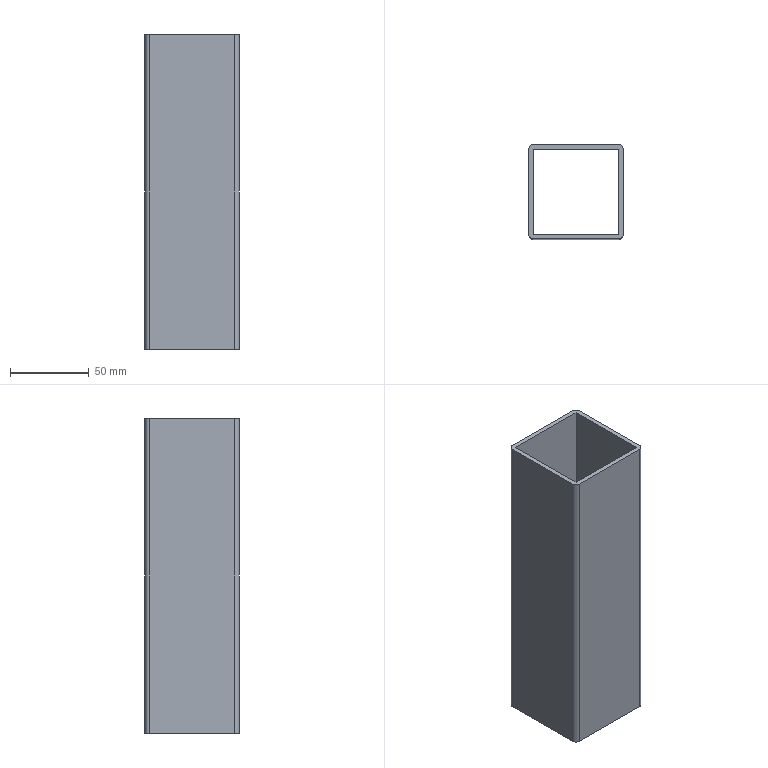Part | STEP file | X77-03109 | 1 solid | 14 faces | box 60 x 60 x 200 mm | volume 135255 mm3 | plane 10 | cylinder 4 | commonest cylinder face diameters 6 x4
STEP:
#1=CARTESIAN_POINT('',(0.,3.,200.));
#2=VERTEX_POINT('',#1);
#3=CARTESIAN_POINT('',(3.,0.,200.));
#4=VERTEX_POINT('',#3);
#5=CARTESIAN_POINT('',(3.,3.,200.));
#6=DIRECTION('',(0.,0.,1.));
#7=DIRECTION('',(1.,0.,0.));
#8=AXIS2_PLACEMENT_3D('',#5,#6,#7);
#9=CIRCLE('',#8,3.);
#10=EDGE_CURVE('',#2,#4,#9,.T.);
#11=ORIENTED_EDGE('',*,*,#10,.T.);
#12=CARTESIAN_POINT('',(57.,0.,200.));
#13=VERTEX_POINT('',#12);
#14=CARTESIAN_POINT('',(3.,0.,200.));
#15=DIRECTION('',(1.,0.,0.));
#16=VECTOR('',#15,1000.);
#17=LINE('',#14,#16);
#18=EDGE_CURVE('',#4,#13,#17,.T.);
#19=ORIENTED_EDGE('',*,*,#18,.T.);
#20=CARTESIAN_POINT('',(60.,3.,200.));
#21=VERTEX_POINT('',#20);
#22=CARTESIAN_POINT('',(57.,3.,200.));
#23=DIRECTION('',(0.,0.,1.));
#24=DIRECTION('',(1.,0.,0.));
#25=AXIS2_PLACEMENT_3D('',#22,#23,#24);
#26=CIRCLE('',#25,3.);
#27=EDGE_CURVE('',#13,#21,#26,.T.);
#28=ORIENTED_EDGE('',*,*,#27,.T.);
#29=CARTESIAN_POINT('',(60.,57.,200.));
#30=VERTEX_POINT('',#29);
#31=CARTESIAN_POINT('',(60.,3.,200.));
#32=DIRECTION('',(0.,1.,0.));
#33=VECTOR('',#32,1000.);
#34=LINE('',#31,#33);
#35=EDGE_CURVE('',#21,#30,#34,.T.);
#36=ORIENTED_EDGE('',*,*,#35,.T.);
#37=CARTESIAN_POINT('',(57.,60.,200.));
#38=VERTEX_POINT('',#37);
#39=CARTESIAN_POINT('',(57.,57.,200.));
#40=DIRECTION('',(0.,0.,1.));
#41=DIRECTION('',(1.,0.,0.));
#42=AXIS2_PLACEMENT_3D('',#39,#40,#41);
#43=CIRCLE('',#42,3.);
#44=EDGE_CURVE('',#30,#38,#43,.T.);
#45=ORIENTED_EDGE('',*,*,#44,.T.);
#46=CARTESIAN_POINT('',(3.,60.,200.));
#47=VERTEX_POINT('',#46);
#48=CARTESIAN_POINT('',(3.,60.,200.));
#49=DIRECTION('',(-1.,0.,0.));
#50=VECTOR('',#49,1000.);
#51=LINE('',#48,#50);
#52=EDGE_CURVE('',#38,#47,#51,.T.);
#53=ORIENTED_EDGE('',*,*,#52,.T.);
#54=CARTESIAN_POINT('',(0.,57.,200.));
#55=VERTEX_POINT('',#54);
#56=CARTESIAN_POINT('',(3.,57.,200.));
#57=DIRECTION('',(0.,0.,1.));
#58=DIRECTION('',(1.,0.,0.));
#59=AXIS2_PLACEMENT_3D('',#56,#57,#58);
#60=CIRCLE('',#59,3.);
#61=EDGE_CURVE('',#47,#55,#60,.T.);
#62=ORIENTED_EDGE('',*,*,#61,.T.);
#63=CARTESIAN_POINT('',(0.,3.,200.));
#64=DIRECTION('',(0.,-1.,0.));
#65=VECTOR('',#64,1000.);
#66=LINE('',#63,#65);
#67=EDGE_CURVE('',#55,#2,#66,.T.);
#68=ORIENTED_EDGE('',*,*,#67,.T.);
#69=EDGE_LOOP('',(#11,#19,#28,#36,#45,#53,#62,#68));
#70=FACE_OUTER_BOUND('',#69,.T.);
#71=CARTESIAN_POINT('',(3.,3.,200.));
#72=VERTEX_POINT('',#71);
#73=CARTESIAN_POINT('',(57.,3.,200.));
#74=VERTEX_POINT('',#73);
#75=CARTESIAN_POINT('',(3.,3.,200.));
#76=DIRECTION('',(1.,0.,0.));
#77=VECTOR('',#76,1000.);
#78=LINE('',#75,#77);
#79=EDGE_CURVE('',#72,#74,#78,.T.);
#80=ORIENTED_EDGE('',*,*,#79,.F.);
#81=CARTESIAN_POINT('',(3.,57.,200.));
#82=VERTEX_POINT('',#81);
#83=CARTESIAN_POINT('',(3.,3.,200.));
#84=DIRECTION('',(0.,-1.,0.));
#85=VECTOR('',#84,1000.);
#86=LINE('',#83,#85);
#87=EDGE_CURVE('',#82,#72,#86,.T.);
#88=ORIENTED_EDGE('',*,*,#87,.F.);
#89=CARTESIAN_POINT('',(57.,57.,200.));
#90=VERTEX_POINT('',#89);
#91=CARTESIAN_POINT('',(3.,57.,200.));
#92=DIRECTION('',(-1.,0.,0.));
#93=VECTOR('',#92,1000.);
#94=LINE('',#91,#93);
#95=EDGE_CURVE('',#90,#82,#94,.T.);
#96=ORIENTED_EDGE('',*,*,#95,.F.);
#97=CARTESIAN_POINT('',(57.,3.,200.));
#98=DIRECTION('',(0.,1.,0.));
#99=VECTOR('',#98,1000.);
#100=LINE('',#97,#99);
#101=EDGE_CURVE('',#74,#90,#100,.T.);
#102=ORIENTED_EDGE('',*,*,#101,.F.);
#103=EDGE_LOOP('',(#80,#88,#96,#102));
#104=FACE_BOUND('',#103,.T.);
#105=CARTESIAN_POINT('',(3.,3.,200.));
#106=DIRECTION('',(0.,0.,1.));
#107=DIRECTION('',(1.,0.,0.));
#108=AXIS2_PLACEMENT_3D('',#105,#106,#107);
#109=PLANE('',#108);
#110=ADVANCED_FACE('',(#70,#104),#109,.T.);
#111=CARTESIAN_POINT('',(0.,3.,0.));
#112=VERTEX_POINT('',#111);
#113=CARTESIAN_POINT('',(3.,0.,0.));
#114=VERTEX_POINT('',#113);
#115=CARTESIAN_POINT('',(3.,3.,0.));
#116=DIRECTION('',(0.,0.,1.));
#117=DIRECTION('',(1.,0.,0.));
#118=AXIS2_PLACEMENT_3D('',#115,#116,#117);
#119=CIRCLE('',#118,3.);
#120=EDGE_CURVE('',#112,#114,#119,.T.);
#121=ORIENTED_EDGE('',*,*,#120,.F.);
#122=CARTESIAN_POINT('',(0.,57.,0.));
#123=VERTEX_POINT('',#122);
#124=CARTESIAN_POINT('',(0.,3.,0.));
#125=DIRECTION('',(0.,-1.,0.));
#126=VECTOR('',#125,1000.);
#127=LINE('',#124,#126);
#128=EDGE_CURVE('',#123,#112,#127,.T.);
#129=ORIENTED_EDGE('',*,*,#128,.F.);
#130=CARTESIAN_POINT('',(3.,60.,0.));
#131=VERTEX_POINT('',#130);
#132=CARTESIAN_POINT('',(3.,57.,0.));
#133=DIRECTION('',(0.,0.,1.));
#134=DIRECTION('',(1.,0.,0.));
#135=AXIS2_PLACEMENT_3D('',#132,#133,#134);
#136=CIRCLE('',#135,3.);
#137=EDGE_CURVE('',#131,#123,#136,.T.);
#138=ORIENTED_EDGE('',*,*,#137,.F.);
#139=CARTESIAN_POINT('',(57.,60.,0.));
#140=VERTEX_POINT('',#139);
#141=CARTESIAN_POINT('',(3.,60.,0.));
#142=DIRECTION('',(-1.,0.,0.));
#143=VECTOR('',#142,1000.);
#144=LINE('',#141,#143);
#145=EDGE_CURVE('',#140,#131,#144,.T.);
#146=ORIENTED_EDGE('',*,*,#145,.F.);
#147=CARTESIAN_POINT('',(60.,57.,0.));
#148=VERTEX_POINT('',#147);
#149=CARTESIAN_POINT('',(57.,57.,0.));
#150=DIRECTION('',(0.,0.,1.));
#151=DIRECTION('',(1.,0.,0.));
#152=AXIS2_PLACEMENT_3D('',#149,#150,#151);
#153=CIRCLE('',#152,3.);
#154=EDGE_CURVE('',#148,#140,#153,.T.);
#155=ORIENTED_EDGE('',*,*,#154,.F.);
#156=CARTESIAN_POINT('',(60.,3.,0.));
#157=VERTEX_POINT('',#156);
#158=CARTESIAN_POINT('',(60.,3.,0.));
#159=DIRECTION('',(0.,1.,0.));
#160=VECTOR('',#159,1000.);
#161=LINE('',#158,#160);
#162=EDGE_CURVE('',#157,#148,#161,.T.);
#163=ORIENTED_EDGE('',*,*,#162,.F.);
#164=CARTESIAN_POINT('',(57.,0.,0.));
#165=VERTEX_POINT('',#164);
#166=CARTESIAN_POINT('',(57.,3.,0.));
#167=DIRECTION('',(0.,0.,1.));
#168=DIRECTION('',(1.,0.,0.));
#169=AXIS2_PLACEMENT_3D('',#166,#167,#168);
#170=CIRCLE('',#169,3.);
#171=EDGE_CURVE('',#165,#157,#170,.T.);
#172=ORIENTED_EDGE('',*,*,#171,.F.);
#173=CARTESIAN_POINT('',(3.,0.,0.));
#174=DIRECTION('',(1.,0.,0.));
#175=VECTOR('',#174,1000.);
#176=LINE('',#173,#175);
#177=EDGE_CURVE('',#114,#165,#176,.T.);
#178=ORIENTED_EDGE('',*,*,#177,.F.);
#179=EDGE_LOOP('',(#121,#129,#138,#146,#155,#163,#172,#178));
#180=FACE_OUTER_BOUND('',#179,.T.);
#181=CARTESIAN_POINT('',(3.,57.,0.));
#182=VERTEX_POINT('',#181);
#183=CARTESIAN_POINT('',(3.,3.,0.));
#184=VERTEX_POINT('',#183);
#185=CARTESIAN_POINT('',(3.,3.,0.));
#186=DIRECTION('',(0.,-1.,0.));
#187=VECTOR('',#186,1000.);
#188=LINE('',#185,#187);
#189=EDGE_CURVE('',#182,#184,#188,.T.);
#190=ORIENTED_EDGE('',*,*,#189,.T.);
#191=CARTESIAN_POINT('',(57.,3.,0.));
#192=VERTEX_POINT('',#191);
#193=CARTESIAN_POINT('',(3.,3.,0.));
#194=DIRECTION('',(1.,0.,0.));
#195=VECTOR('',#194,1000.);
#196=LINE('',#193,#195);
#197=EDGE_CURVE('',#184,#192,#196,.T.);
#198=ORIENTED_EDGE('',*,*,#197,.T.);
#199=CARTESIAN_POINT('',(57.,57.,0.));
#200=VERTEX_POINT('',#199);
#201=CARTESIAN_POINT('',(57.,3.,0.));
#202=DIRECTION('',(0.,1.,0.));
#203=VECTOR('',#202,1000.);
#204=LINE('',#201,#203);
#205=EDGE_CURVE('',#192,#200,#204,.T.);
#206=ORIENTED_EDGE('',*,*,#205,.T.);
#207=CARTESIAN_POINT('',(3.,57.,0.));
#208=DIRECTION('',(-1.,0.,0.));
#209=VECTOR('',#208,1000.);
#210=LINE('',#207,#209);
#211=EDGE_CURVE('',#200,#182,#210,.T.);
#212=ORIENTED_EDGE('',*,*,#211,.T.);
#213=EDGE_LOOP('',(#190,#198,#206,#212));
#214=FACE_BOUND('',#213,.T.);
#215=CARTESIAN_POINT('',(3.,3.,0.));
#216=DIRECTION('',(0.,0.,1.));
#217=DIRECTION('',(1.,0.,0.));
#218=AXIS2_PLACEMENT_3D('',#215,#216,#217);
#219=PLANE('',#218);
#220=ADVANCED_FACE('',(#180,#214),#219,.F.);
#221=ORIENTED_EDGE('',*,*,#120,.T.);
#222=CARTESIAN_POINT('',(3.,0.,200.));
#223=DIRECTION('',(0.,0.,-1.));
#224=VECTOR('',#223,1000.);
#225=LINE('',#222,#224);
#226=EDGE_CURVE('',#4,#114,#225,.T.);
#227=ORIENTED_EDGE('',*,*,#226,.F.);
#228=ORIENTED_EDGE('',*,*,#10,.F.);
#229=CARTESIAN_POINT('',(0.,3.,200.));
#230=DIRECTION('',(0.,0.,-1.));
#231=VECTOR('',#230,1000.);
#232=LINE('',#229,#231);
#233=EDGE_CURVE('',#2,#112,#232,.T.);
#234=ORIENTED_EDGE('',*,*,#233,.T.);
#235=EDGE_LOOP('',(#221,#227,#228,#234));
#236=FACE_OUTER_BOUND('',#235,.T.);
#237=CARTESIAN_POINT('',(3.,3.,200.));
#238=DIRECTION('',(0.,0.,-1.));
#239=DIRECTION('',(-1.,0.,0.));
#240=AXIS2_PLACEMENT_3D('',#237,#238,#239);
#241=CYLINDRICAL_SURFACE('',#240,3.);
#242=ADVANCED_FACE('',(#236),#241,.T.);
#243=ORIENTED_EDGE('',*,*,#177,.T.);
#244=CARTESIAN_POINT('',(57.,0.,200.));
#245=DIRECTION('',(0.,0.,-1.));
#246=VECTOR('',#245,1000.);
#247=LINE('',#244,#246);
#248=EDGE_CURVE('',#13,#165,#247,.T.);
#249=ORIENTED_EDGE('',*,*,#248,.F.);
#250=ORIENTED_EDGE('',*,*,#18,.F.);
#251=ORIENTED_EDGE('',*,*,#226,.T.);
#252=EDGE_LOOP('',(#243,#249,#250,#251));
#253=FACE_OUTER_BOUND('',#252,.T.);
#254=CARTESIAN_POINT('',(3.,0.,200.));
#255=DIRECTION('',(0.,1.,0.));
#256=DIRECTION('',(0.,0.,1.));
#257=AXIS2_PLACEMENT_3D('',#254,#255,#256);
#258=PLANE('',#257);
#259=ADVANCED_FACE('',(#253),#258,.F.);
#260=ORIENTED_EDGE('',*,*,#171,.T.);
#261=CARTESIAN_POINT('',(60.,3.,200.));
#262=DIRECTION('',(0.,0.,-1.));
#263=VECTOR('',#262,1000.);
#264=LINE('',#261,#263);
#265=EDGE_CURVE('',#21,#157,#264,.T.);
#266=ORIENTED_EDGE('',*,*,#265,.F.);
#267=ORIENTED_EDGE('',*,*,#27,.F.);
#268=ORIENTED_EDGE('',*,*,#248,.T.);
#269=EDGE_LOOP('',(#260,#266,#267,#268));
#270=FACE_OUTER_BOUND('',#269,.T.);
#271=CARTESIAN_POINT('',(57.,3.,200.));
#272=DIRECTION('',(0.,0.,-1.));
#273=DIRECTION('',(-1.,0.,0.));
#274=AXIS2_PLACEMENT_3D('',#271,#272,#273);
#275=CYLINDRICAL_SURFACE('',#274,3.);
#276=ADVANCED_FACE('',(#270),#275,.T.);
#277=ORIENTED_EDGE('',*,*,#162,.T.);
#278=CARTESIAN_POINT('',(60.,57.,200.));
#279=DIRECTION('',(0.,0.,-1.));
#280=VECTOR('',#279,1000.);
#281=LINE('',#278,#280);
#282=EDGE_CURVE('',#30,#148,#281,.T.);
#283=ORIENTED_EDGE('',*,*,#282,.F.);
#284=ORIENTED_EDGE('',*,*,#35,.F.);
#285=ORIENTED_EDGE('',*,*,#265,.T.);
#286=EDGE_LOOP('',(#277,#283,#284,#285));
#287=FACE_OUTER_BOUND('',#286,.T.);
#288=CARTESIAN_POINT('',(60.,3.,200.));
#289=DIRECTION('',(-1.,0.,0.));
#290=DIRECTION('',(0.,0.,1.));
#291=AXIS2_PLACEMENT_3D('',#288,#289,#290);
#292=PLANE('',#291);
#293=ADVANCED_FACE('',(#287),#292,.F.);
#294=ORIENTED_EDGE('',*,*,#154,.T.);
#295=CARTESIAN_POINT('',(57.,60.,200.));
#296=DIRECTION('',(0.,0.,-1.));
#297=VECTOR('',#296,1000.);
#298=LINE('',#295,#297);
#299=EDGE_CURVE('',#38,#140,#298,.T.);
#300=ORIENTED_EDGE('',*,*,#299,.F.);
#301=ORIENTED_EDGE('',*,*,#44,.F.);
#302=ORIENTED_EDGE('',*,*,#282,.T.);
#303=EDGE_LOOP('',(#294,#300,#301,#302));
#304=FACE_OUTER_BOUND('',#303,.T.);
#305=CARTESIAN_POINT('',(57.,57.,200.));
#306=DIRECTION('',(0.,0.,-1.));
#307=DIRECTION('',(-1.,0.,0.));
#308=AXIS2_PLACEMENT_3D('',#305,#306,#307);
#309=CYLINDRICAL_SURFACE('',#308,3.);
#310=ADVANCED_FACE('',(#304),#309,.T.);
#311=ORIENTED_EDGE('',*,*,#145,.T.);
#312=CARTESIAN_POINT('',(3.,60.,200.));
#313=DIRECTION('',(0.,0.,-1.));
#314=VECTOR('',#313,1000.);
#315=LINE('',#312,#314);
#316=EDGE_CURVE('',#47,#131,#315,.T.);
#317=ORIENTED_EDGE('',*,*,#316,.F.);
#318=ORIENTED_EDGE('',*,*,#52,.F.);
#319=ORIENTED_EDGE('',*,*,#299,.T.);
#320=EDGE_LOOP('',(#311,#317,#318,#319));
#321=FACE_OUTER_BOUND('',#320,.T.);
#322=CARTESIAN_POINT('',(3.,60.,200.));
#323=DIRECTION('',(0.,-1.,0.));
#324=DIRECTION('',(0.,0.,-1.));
#325=AXIS2_PLACEMENT_3D('',#322,#323,#324);
#326=PLANE('',#325);
#327=ADVANCED_FACE('',(#321),#326,.F.);
#328=ORIENTED_EDGE('',*,*,#137,.T.);
#329=CARTESIAN_POINT('',(0.,57.,200.));
#330=DIRECTION('',(0.,0.,-1.));
#331=VECTOR('',#330,1000.);
#332=LINE('',#329,#331);
#333=EDGE_CURVE('',#55,#123,#332,.T.);
#334=ORIENTED_EDGE('',*,*,#333,.F.);
#335=ORIENTED_EDGE('',*,*,#61,.F.);
#336=ORIENTED_EDGE('',*,*,#316,.T.);
#337=EDGE_LOOP('',(#328,#334,#335,#336));
#338=FACE_OUTER_BOUND('',#337,.T.);
#339=CARTESIAN_POINT('',(3.,57.,200.));
#340=DIRECTION('',(0.,0.,-1.));
#341=DIRECTION('',(-1.,0.,0.));
#342=AXIS2_PLACEMENT_3D('',#339,#340,#341);
#343=CYLINDRICAL_SURFACE('',#342,3.);
#344=ADVANCED_FACE('',(#338),#343,.T.);
#345=ORIENTED_EDGE('',*,*,#128,.T.);
#346=ORIENTED_EDGE('',*,*,#233,.F.);
#347=ORIENTED_EDGE('',*,*,#67,.F.);
#348=ORIENTED_EDGE('',*,*,#333,.T.);
#349=EDGE_LOOP('',(#345,#346,#347,#348));
#350=FACE_OUTER_BOUND('',#349,.T.);
#351=CARTESIAN_POINT('',(0.,3.,200.));
#352=DIRECTION('',(1.,0.,0.));
#353=DIRECTION('',(0.,0.,-1.));
#354=AXIS2_PLACEMENT_3D('',#351,#352,#353);
#355=PLANE('',#354);
#356=ADVANCED_FACE('',(#350),#355,.F.);
#357=ORIENTED_EDGE('',*,*,#189,.F.);
#358=CARTESIAN_POINT('',(3.,57.,200.));
#359=DIRECTION('',(0.,0.,-1.));
#360=VECTOR('',#359,1000.);
#361=LINE('',#358,#360);
#362=EDGE_CURVE('',#82,#182,#361,.T.);
#363=ORIENTED_EDGE('',*,*,#362,.F.);
#364=ORIENTED_EDGE('',*,*,#87,.T.);
#365=CARTESIAN_POINT('',(3.,3.,200.));
#366=DIRECTION('',(0.,0.,-1.));
#367=VECTOR('',#366,1000.);
#368=LINE('',#365,#367);
#369=EDGE_CURVE('',#72,#184,#368,.T.);
#370=ORIENTED_EDGE('',*,*,#369,.T.);
#371=EDGE_LOOP('',(#357,#363,#364,#370));
#372=FACE_OUTER_BOUND('',#371,.T.);
#373=CARTESIAN_POINT('',(3.,3.,200.));
#374=DIRECTION('',(1.,0.,0.));
#375=DIRECTION('',(0.,0.,-1.));
#376=AXIS2_PLACEMENT_3D('',#373,#374,#375);
#377=PLANE('',#376);
#378=ADVANCED_FACE('',(#372),#377,.T.);
#379=ORIENTED_EDGE('',*,*,#197,.F.);
#380=ORIENTED_EDGE('',*,*,#369,.F.);
#381=ORIENTED_EDGE('',*,*,#79,.T.);
#382=CARTESIAN_POINT('',(57.,3.,200.));
#383=DIRECTION('',(0.,0.,-1.));
#384=VECTOR('',#383,1000.);
#385=LINE('',#382,#384);
#386=EDGE_CURVE('',#74,#192,#385,.T.);
#387=ORIENTED_EDGE('',*,*,#386,.T.);
#388=EDGE_LOOP('',(#379,#380,#381,#387));
#389=FACE_OUTER_BOUND('',#388,.T.);
#390=CARTESIAN_POINT('',(3.,3.,200.));
#391=DIRECTION('',(0.,1.,0.));
#392=DIRECTION('',(0.,0.,1.));
#393=AXIS2_PLACEMENT_3D('',#390,#391,#392);
#394=PLANE('',#393);
#395=ADVANCED_FACE('',(#389),#394,.T.);
#396=ORIENTED_EDGE('',*,*,#205,.F.);
#397=ORIENTED_EDGE('',*,*,#386,.F.);
#398=ORIENTED_EDGE('',*,*,#101,.T.);
#399=CARTESIAN_POINT('',(57.,57.,200.));
#400=DIRECTION('',(0.,0.,-1.));
#401=VECTOR('',#400,1000.);
#402=LINE('',#399,#401);
#403=EDGE_CURVE('',#90,#200,#402,.T.);
#404=ORIENTED_EDGE('',*,*,#403,.T.);
#405=EDGE_LOOP('',(#396,#397,#398,#404));
#406=FACE_OUTER_BOUND('',#405,.T.);
#407=CARTESIAN_POINT('',(57.,3.,200.));
#408=DIRECTION('',(-1.,0.,0.));
#409=DIRECTION('',(0.,0.,1.));
#410=AXIS2_PLACEMENT_3D('',#407,#408,#409);
#411=PLANE('',#410);
#412=ADVANCED_FACE('',(#406),#411,.T.);
#413=ORIENTED_EDGE('',*,*,#211,.F.);
#414=ORIENTED_EDGE('',*,*,#403,.F.);
#415=ORIENTED_EDGE('',*,*,#95,.T.);
#416=ORIENTED_EDGE('',*,*,#362,.T.);
#417=EDGE_LOOP('',(#413,#414,#415,#416));
#418=FACE_OUTER_BOUND('',#417,.T.);
#419=CARTESIAN_POINT('',(3.,57.,200.));
#420=DIRECTION('',(0.,-1.,0.));
#421=DIRECTION('',(0.,0.,-1.));
#422=AXIS2_PLACEMENT_3D('',#419,#420,#421);
#423=PLANE('',#422);
#424=ADVANCED_FACE('',(#418),#423,.T.);
#425=CLOSED_SHELL('',(#110,#220,#242,#259,#276,#293,#310,#327,#344,#356,#378,#395,#412,#424));
#426=MANIFOLD_SOLID_BREP('',#425);
#427=CARTESIAN_POINT('',(0.,0.,0.));
#428=DIRECTION('',(0.,0.,1.));
#429=DIRECTION('',(1.,0.,0.));
#430=AXIS2_PLACEMENT_3D('',#427,#428,#429);
#431=(LENGTH_UNIT()NAMED_UNIT(*)SI_UNIT(.MILLI.,.METRE.));
#432=UNCERTAINTY_MEASURE_WITH_UNIT(LENGTH_MEASURE(0.00001),#431,'','');
#433=(NAMED_UNIT(*)PLANE_ANGLE_UNIT()SI_UNIT($,.RADIAN.));
#434=(NAMED_UNIT(*)SI_UNIT($,.STERADIAN.)SOLID_ANGLE_UNIT());
#435=(GEOMETRIC_REPRESENTATION_CONTEXT(3)GLOBAL_UNCERTAINTY_ASSIGNED_CONTEXT((#432))GLOBAL_UNIT_ASSIGNED_CONTEXT((#431,#433,#434))REPRESENTATION_CONTEXT('',''));
#436=ADVANCED_BREP_SHAPE_REPRESENTATION('',(#426,#430),#435);